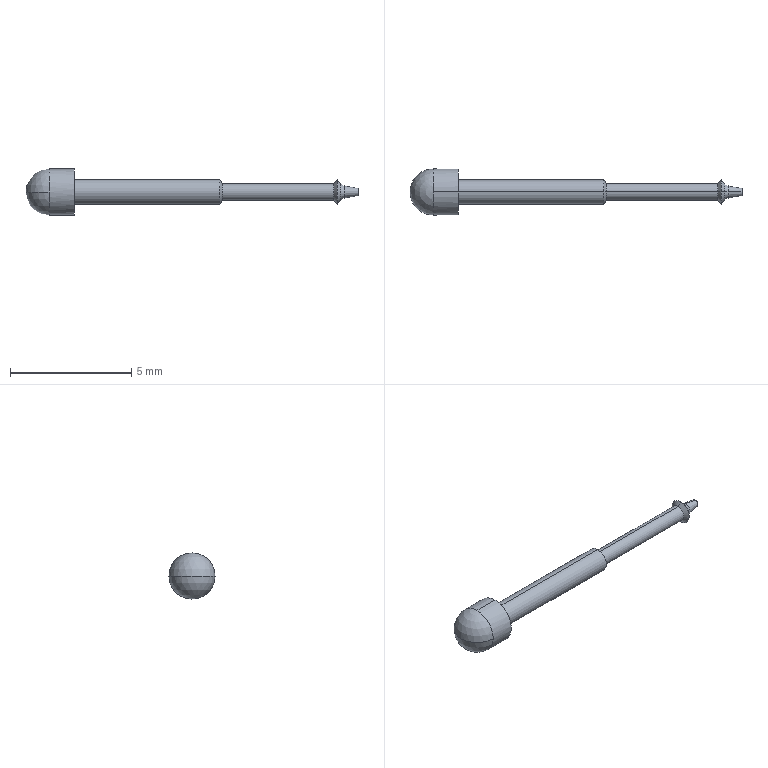Part | STEP file | Shape_NP604_B | 1 solid | 20 faces | box 13.7 x 1.9 x 1.9 mm | volume 11.415 mm3 | cone 10 | cylinder 6 | sphere 2 | plane 2 | commonest cylinder face diameters 0.667 x2 1 x2 1.9 x2
STEP:
#1=CARTESIAN_POINT('',(0.95,0.,-0.95));
#2=VERTEX_POINT('',#1);
#3=CARTESIAN_POINT('',(0.95,-0.95,0.));
#4=VERTEX_POINT('',#3);
#5=CARTESIAN_POINT('',(0.95,0.,0.));
#6=DIRECTION('',(-1.,0.,0.));
#7=DIRECTION('',(0.,0.,1.));
#8=AXIS2_PLACEMENT_3D('',#5,#6,#7);
#9=CIRCLE('',#8,0.95);
#10=EDGE_CURVE('',#2,#4,#9,.T.);
#11=ORIENTED_EDGE('',*,*,#10,.T.);
#12=CARTESIAN_POINT('',(0.,0.,0.));
#13=VERTEX_POINT('',#12);
#14=CARTESIAN_POINT('',(0.95,0.,0.));
#15=DIRECTION('',(0.,0.,-1.));
#16=DIRECTION('',(0.,1.,0.));
#17=AXIS2_PLACEMENT_3D('',#14,#15,#16);
#18=CIRCLE('',#17,0.95);
#19=EDGE_CURVE('',#4,#13,#18,.T.);
#20=ORIENTED_EDGE('',*,*,#19,.T.);
#21=CARTESIAN_POINT('',(0.95,0.95,0.));
#22=VERTEX_POINT('',#21);
#23=CARTESIAN_POINT('',(0.95,0.,0.));
#24=DIRECTION('',(0.,0.,1.));
#25=DIRECTION('',(1.,0.,0.));
#26=AXIS2_PLACEMENT_3D('',#23,#24,#25);
#27=CIRCLE('',#26,0.95);
#28=EDGE_CURVE('',#22,#13,#27,.T.);
#29=ORIENTED_EDGE('',*,*,#28,.F.);
#30=CARTESIAN_POINT('',(0.95,0.,0.));
#31=DIRECTION('',(-1.,0.,0.));
#32=DIRECTION('',(0.,0.,1.));
#33=AXIS2_PLACEMENT_3D('',#30,#31,#32);
#34=CIRCLE('',#33,0.95);
#35=EDGE_CURVE('',#22,#2,#34,.T.);
#36=ORIENTED_EDGE('',*,*,#35,.T.);
#37=EDGE_LOOP('',(#11,#20,#29,#36));
#38=FACE_OUTER_BOUND('',#37,.T.);
#39=CARTESIAN_POINT('',(0.95,0.,0.));
#40=DIRECTION('',(0.,0.,-1.));
#41=DIRECTION('',(0.,1.,0.));
#42=AXIS2_PLACEMENT_3D('',#39,#40,#41);
#43=SPHERICAL_SURFACE('',#42,0.95);
#44=ADVANCED_FACE('',(#38),#43,.T.);
#45=CARTESIAN_POINT('',(13.7,0.,0.1484));
#46=VERTEX_POINT('',#45);
#47=CARTESIAN_POINT('',(13.7,0.,-0.1484));
#48=VERTEX_POINT('',#47);
#49=CARTESIAN_POINT('',(13.7,0.,0.));
#50=DIRECTION('',(-1.,0.,0.));
#51=DIRECTION('',(0.,0.,1.));
#52=AXIS2_PLACEMENT_3D('',#49,#50,#51);
#53=CIRCLE('',#52,0.1484);
#54=EDGE_CURVE('',#46,#48,#53,.T.);
#55=ORIENTED_EDGE('',*,*,#54,.T.);
#56=CARTESIAN_POINT('',(13.124,0.,-0.25));
#57=VERTEX_POINT('',#56);
#58=CARTESIAN_POINT('',(13.7,0.,-0.1484));
#59=DIRECTION('',(-0.9848,0.,-0.1736));
#60=VECTOR('',#59,1000.);
#61=LINE('',#58,#60);
#62=EDGE_CURVE('',#48,#57,#61,.T.);
#63=ORIENTED_EDGE('',*,*,#62,.T.);
#64=CARTESIAN_POINT('',(13.124,0.,0.25));
#65=VERTEX_POINT('',#64);
#66=CARTESIAN_POINT('',(13.124,0.,0.));
#67=DIRECTION('',(-1.,0.,0.));
#68=DIRECTION('',(0.,0.,1.));
#69=AXIS2_PLACEMENT_3D('',#66,#67,#68);
#70=CIRCLE('',#69,0.25);
#71=EDGE_CURVE('',#65,#57,#70,.T.);
#72=ORIENTED_EDGE('',*,*,#71,.F.);
#73=CARTESIAN_POINT('',(13.7,0.,0.1484));
#74=DIRECTION('',(-0.9848,0.,0.1736));
#75=VECTOR('',#74,1000.);
#76=LINE('',#73,#75);
#77=EDGE_CURVE('',#46,#65,#76,.T.);
#78=ORIENTED_EDGE('',*,*,#77,.F.);
#79=EDGE_LOOP('',(#55,#63,#72,#78));
#80=FACE_OUTER_BOUND('',#79,.T.);
#81=CARTESIAN_POINT('',(13.7,0.,0.));
#82=DIRECTION('',(-1.,0.,0.));
#83=DIRECTION('',(0.,0.,1.));
#84=AXIS2_PLACEMENT_3D('',#81,#82,#83);
#85=CONICAL_SURFACE('',#84,0.1484,0.1745);
#86=ADVANCED_FACE('',(#80),#85,.T.);
#87=ORIENTED_EDGE('',*,*,#71,.T.);
#88=CARTESIAN_POINT('',(12.98,0.,-0.3333));
#89=VERTEX_POINT('',#88);
#90=CARTESIAN_POINT('',(13.124,0.,-0.25));
#91=DIRECTION('',(-0.866,0.,-0.5));
#92=VECTOR('',#91,1000.);
#93=LINE('',#90,#92);
#94=EDGE_CURVE('',#57,#89,#93,.T.);
#95=ORIENTED_EDGE('',*,*,#94,.T.);
#96=CARTESIAN_POINT('',(12.98,0.,0.3333));
#97=VERTEX_POINT('',#96);
#98=CARTESIAN_POINT('',(12.98,0.,0.));
#99=DIRECTION('',(-1.,0.,0.));
#100=DIRECTION('',(0.,0.,1.));
#101=AXIS2_PLACEMENT_3D('',#98,#99,#100);
#102=CIRCLE('',#101,0.3333);
#103=EDGE_CURVE('',#97,#89,#102,.T.);
#104=ORIENTED_EDGE('',*,*,#103,.F.);
#105=CARTESIAN_POINT('',(13.124,0.,0.25));
#106=DIRECTION('',(-0.866,0.,0.5));
#107=VECTOR('',#106,1000.);
#108=LINE('',#105,#107);
#109=EDGE_CURVE('',#65,#97,#108,.T.);
#110=ORIENTED_EDGE('',*,*,#109,.F.);
#111=EDGE_LOOP('',(#87,#95,#104,#110));
#112=FACE_OUTER_BOUND('',#111,.T.);
#113=CARTESIAN_POINT('',(13.124,0.,0.));
#114=DIRECTION('',(-1.,0.,0.));
#115=DIRECTION('',(0.,0.,1.));
#116=AXIS2_PLACEMENT_3D('',#113,#114,#115);
#117=CONICAL_SURFACE('',#116,0.25,0.5236);
#118=ADVANCED_FACE('',(#112),#117,.T.);
#119=ORIENTED_EDGE('',*,*,#103,.T.);
#120=CARTESIAN_POINT('',(12.837,0.,-0.5033));
#121=VERTEX_POINT('',#120);
#122=CARTESIAN_POINT('',(12.98,0.,-0.3333));
#123=DIRECTION('',(-0.6428,0.,-0.766));
#124=VECTOR('',#123,1000.);
#125=LINE('',#122,#124);
#126=EDGE_CURVE('',#89,#121,#125,.T.);
#127=ORIENTED_EDGE('',*,*,#126,.T.);
#128=CARTESIAN_POINT('',(12.837,0.,0.5033));
#129=VERTEX_POINT('',#128);
#130=CARTESIAN_POINT('',(12.837,0.,0.));
#131=DIRECTION('',(-1.,0.,0.));
#132=DIRECTION('',(0.,0.,1.));
#133=AXIS2_PLACEMENT_3D('',#130,#131,#132);
#134=CIRCLE('',#133,0.5033);
#135=EDGE_CURVE('',#129,#121,#134,.T.);
#136=ORIENTED_EDGE('',*,*,#135,.F.);
#137=CARTESIAN_POINT('',(12.98,0.,0.3333));
#138=DIRECTION('',(-0.6428,0.,0.766));
#139=VECTOR('',#138,1000.);
#140=LINE('',#137,#139);
#141=EDGE_CURVE('',#97,#129,#140,.T.);
#142=ORIENTED_EDGE('',*,*,#141,.F.);
#143=EDGE_LOOP('',(#119,#127,#136,#142));
#144=FACE_OUTER_BOUND('',#143,.T.);
#145=CARTESIAN_POINT('',(12.98,0.,0.));
#146=DIRECTION('',(-1.,0.,0.));
#147=DIRECTION('',(0.,0.,1.));
#148=AXIS2_PLACEMENT_3D('',#145,#146,#147);
#149=CONICAL_SURFACE('',#148,0.3333,0.8727);
#150=ADVANCED_FACE('',(#144),#149,.T.);
#151=CARTESIAN_POINT('',(12.694,0.,0.3333));
#152=VERTEX_POINT('',#151);
#153=CARTESIAN_POINT('',(12.694,0.,-0.3333));
#154=VERTEX_POINT('',#153);
#155=CARTESIAN_POINT('',(12.694,0.,0.));
#156=DIRECTION('',(-1.,0.,0.));
#157=DIRECTION('',(0.,0.,1.));
#158=AXIS2_PLACEMENT_3D('',#155,#156,#157);
#159=CIRCLE('',#158,0.3333);
#160=EDGE_CURVE('',#152,#154,#159,.T.);
#161=ORIENTED_EDGE('',*,*,#160,.F.);
#162=CARTESIAN_POINT('',(12.837,0.,0.5033));
#163=DIRECTION('',(0.6428,0.,0.766));
#164=VECTOR('',#163,1000.);
#165=LINE('',#162,#164);
#166=EDGE_CURVE('',#152,#129,#165,.T.);
#167=ORIENTED_EDGE('',*,*,#166,.T.);
#168=ORIENTED_EDGE('',*,*,#135,.T.);
#169=CARTESIAN_POINT('',(12.837,0.,-0.5033));
#170=DIRECTION('',(0.6428,0.,-0.766));
#171=VECTOR('',#170,1000.);
#172=LINE('',#169,#171);
#173=EDGE_CURVE('',#154,#121,#172,.T.);
#174=ORIENTED_EDGE('',*,*,#173,.F.);
#175=EDGE_LOOP('',(#161,#167,#168,#174));
#176=FACE_OUTER_BOUND('',#175,.T.);
#177=CARTESIAN_POINT('',(12.837,0.,0.));
#178=DIRECTION('',(1.,0.,0.));
#179=DIRECTION('',(0.,0.,-1.));
#180=AXIS2_PLACEMENT_3D('',#177,#178,#179);
#181=CONICAL_SURFACE('',#180,0.5033,0.8727);
#182=ADVANCED_FACE('',(#176),#181,.T.);
#183=ORIENTED_EDGE('',*,*,#160,.T.);
#184=CARTESIAN_POINT('',(8.096,0.,-0.3333));
#185=VERTEX_POINT('',#184);
#186=CARTESIAN_POINT('',(13.7,0.,-0.3333));
#187=DIRECTION('',(-1.,0.,0.));
#188=VECTOR('',#187,1000.);
#189=LINE('',#186,#188);
#190=EDGE_CURVE('',#154,#185,#189,.T.);
#191=ORIENTED_EDGE('',*,*,#190,.T.);
#192=CARTESIAN_POINT('',(8.096,0.,0.3333));
#193=VERTEX_POINT('',#192);
#194=CARTESIAN_POINT('',(8.096,0.,0.));
#195=DIRECTION('',(-1.,0.,0.));
#196=DIRECTION('',(0.,0.,1.));
#197=AXIS2_PLACEMENT_3D('',#194,#195,#196);
#198=CIRCLE('',#197,0.3333);
#199=EDGE_CURVE('',#193,#185,#198,.T.);
#200=ORIENTED_EDGE('',*,*,#199,.F.);
#201=CARTESIAN_POINT('',(13.7,0.,0.3333));
#202=DIRECTION('',(-1.,0.,0.));
#203=VECTOR('',#202,1000.);
#204=LINE('',#201,#203);
#205=EDGE_CURVE('',#152,#193,#204,.T.);
#206=ORIENTED_EDGE('',*,*,#205,.F.);
#207=EDGE_LOOP('',(#183,#191,#200,#206));
#208=FACE_OUTER_BOUND('',#207,.T.);
#209=CARTESIAN_POINT('',(13.7,0.,0.));
#210=DIRECTION('',(-1.,0.,0.));
#211=DIRECTION('',(0.,0.,1.));
#212=AXIS2_PLACEMENT_3D('',#209,#210,#211);
#213=CYLINDRICAL_SURFACE('',#212,0.3333);
#214=ADVANCED_FACE('',(#208),#213,.T.);
#215=ORIENTED_EDGE('',*,*,#199,.T.);
#216=CARTESIAN_POINT('',(8.,0.,-0.5));
#217=VERTEX_POINT('',#216);
#218=CARTESIAN_POINT('',(8.096,0.,-0.3333));
#219=DIRECTION('',(-0.5,0.,-0.866));
#220=VECTOR('',#219,1000.);
#221=LINE('',#218,#220);
#222=EDGE_CURVE('',#185,#217,#221,.T.);
#223=ORIENTED_EDGE('',*,*,#222,.T.);
#224=CARTESIAN_POINT('',(8.,0.,0.5));
#225=VERTEX_POINT('',#224);
#226=CARTESIAN_POINT('',(8.,0.,0.));
#227=DIRECTION('',(-1.,0.,0.));
#228=DIRECTION('',(0.,0.,1.));
#229=AXIS2_PLACEMENT_3D('',#226,#227,#228);
#230=CIRCLE('',#229,0.5);
#231=EDGE_CURVE('',#225,#217,#230,.T.);
#232=ORIENTED_EDGE('',*,*,#231,.F.);
#233=CARTESIAN_POINT('',(8.096,0.,0.3333));
#234=DIRECTION('',(-0.5,0.,0.866));
#235=VECTOR('',#234,1000.);
#236=LINE('',#233,#235);
#237=EDGE_CURVE('',#193,#225,#236,.T.);
#238=ORIENTED_EDGE('',*,*,#237,.F.);
#239=EDGE_LOOP('',(#215,#223,#232,#238));
#240=FACE_OUTER_BOUND('',#239,.T.);
#241=CARTESIAN_POINT('',(8.096,0.,0.));
#242=DIRECTION('',(-1.,0.,0.));
#243=DIRECTION('',(0.,0.,1.));
#244=AXIS2_PLACEMENT_3D('',#241,#242,#243);
#245=CONICAL_SURFACE('',#244,0.3333,1.047);
#246=ADVANCED_FACE('',(#240),#245,.T.);
#247=ORIENTED_EDGE('',*,*,#231,.T.);
#248=CARTESIAN_POINT('',(2.,0.,-0.5));
#249=VERTEX_POINT('',#248);
#250=CARTESIAN_POINT('',(13.7,0.,-0.5));
#251=DIRECTION('',(-1.,0.,0.));
#252=VECTOR('',#251,1000.);
#253=LINE('',#250,#252);
#254=EDGE_CURVE('',#217,#249,#253,.T.);
#255=ORIENTED_EDGE('',*,*,#254,.T.);
#256=CARTESIAN_POINT('',(2.,0.,0.5));
#257=VERTEX_POINT('',#256);
#258=CARTESIAN_POINT('',(2.,0.,0.));
#259=DIRECTION('',(-1.,0.,0.));
#260=DIRECTION('',(0.,0.,1.));
#261=AXIS2_PLACEMENT_3D('',#258,#259,#260);
#262=CIRCLE('',#261,0.5);
#263=EDGE_CURVE('',#257,#249,#262,.T.);
#264=ORIENTED_EDGE('',*,*,#263,.F.);
#265=CARTESIAN_POINT('',(13.7,0.,0.5));
#266=DIRECTION('',(-1.,0.,0.));
#267=VECTOR('',#266,1000.);
#268=LINE('',#265,#267);
#269=EDGE_CURVE('',#225,#257,#268,.T.);
#270=ORIENTED_EDGE('',*,*,#269,.F.);
#271=EDGE_LOOP('',(#247,#255,#264,#270));
#272=FACE_OUTER_BOUND('',#271,.T.);
#273=CARTESIAN_POINT('',(13.7,0.,0.));
#274=DIRECTION('',(-1.,0.,0.));
#275=DIRECTION('',(0.,0.,1.));
#276=AXIS2_PLACEMENT_3D('',#273,#274,#275);
#277=CYLINDRICAL_SURFACE('',#276,0.5);
#278=ADVANCED_FACE('',(#272),#277,.T.);
#279=CARTESIAN_POINT('',(2.,0.,0.95));
#280=VERTEX_POINT('',#279);
#281=CARTESIAN_POINT('',(2.,0.,-0.95));
#282=VERTEX_POINT('',#281);
#283=CARTESIAN_POINT('',(2.,0.,0.));
#284=DIRECTION('',(-1.,0.,0.));
#285=DIRECTION('',(0.,0.,1.));
#286=AXIS2_PLACEMENT_3D('',#283,#284,#285);
#287=CIRCLE('',#286,0.95);
#288=EDGE_CURVE('',#280,#282,#287,.T.);
#289=ORIENTED_EDGE('',*,*,#288,.T.);
#290=CARTESIAN_POINT('',(13.7,0.,-0.95));
#291=DIRECTION('',(-1.,0.,0.));
#292=VECTOR('',#291,1000.);
#293=LINE('',#290,#292);
#294=EDGE_CURVE('',#282,#2,#293,.T.);
#295=ORIENTED_EDGE('',*,*,#294,.T.);
#296=ORIENTED_EDGE('',*,*,#35,.F.);
#297=CARTESIAN_POINT('',(0.95,0.,0.95));
#298=VERTEX_POINT('',#297);
#299=CARTESIAN_POINT('',(0.95,0.,0.));
#300=DIRECTION('',(-1.,0.,0.));
#301=DIRECTION('',(0.,0.,1.));
#302=AXIS2_PLACEMENT_3D('',#299,#300,#301);
#303=CIRCLE('',#302,0.95);
#304=EDGE_CURVE('',#298,#22,#303,.T.);
#305=ORIENTED_EDGE('',*,*,#304,.F.);
#306=CARTESIAN_POINT('',(13.7,0.,0.95));
#307=DIRECTION('',(-1.,0.,0.));
#308=VECTOR('',#307,1000.);
#309=LINE('',#306,#308);
#310=EDGE_CURVE('',#280,#298,#309,.T.);
#311=ORIENTED_EDGE('',*,*,#310,.F.);
#312=EDGE_LOOP('',(#289,#295,#296,#305,#311));
#313=FACE_OUTER_BOUND('',#312,.T.);
#314=CARTESIAN_POINT('',(13.7,0.,0.));
#315=DIRECTION('',(-1.,0.,0.));
#316=DIRECTION('',(0.,0.,1.));
#317=AXIS2_PLACEMENT_3D('',#314,#315,#316);
#318=CYLINDRICAL_SURFACE('',#317,0.95);
#319=ADVANCED_FACE('',(#313),#318,.T.);
#320=ORIENTED_EDGE('',*,*,#294,.F.);
#321=CARTESIAN_POINT('',(2.,0.,0.));
#322=DIRECTION('',(-1.,0.,0.));
#323=DIRECTION('',(0.,0.,1.));
#324=AXIS2_PLACEMENT_3D('',#321,#322,#323);
#325=CIRCLE('',#324,0.95);
#326=EDGE_CURVE('',#282,#280,#325,.T.);
#327=ORIENTED_EDGE('',*,*,#326,.T.);
#328=ORIENTED_EDGE('',*,*,#310,.T.);
#329=CARTESIAN_POINT('',(0.95,0.,0.));
#330=DIRECTION('',(-1.,0.,0.));
#331=DIRECTION('',(0.,0.,1.));
#332=AXIS2_PLACEMENT_3D('',#329,#330,#331);
#333=CIRCLE('',#332,0.95);
#334=EDGE_CURVE('',#4,#298,#333,.T.);
#335=ORIENTED_EDGE('',*,*,#334,.F.);
#336=ORIENTED_EDGE('',*,*,#10,.F.);
#337=EDGE_LOOP('',(#320,#327,#328,#335,#336));
#338=FACE_OUTER_BOUND('',#337,.T.);
#339=CARTESIAN_POINT('',(13.7,0.,0.));
#340=DIRECTION('',(-1.,0.,0.));
#341=DIRECTION('',(0.,0.,1.));
#342=AXIS2_PLACEMENT_3D('',#339,#340,#341);
#343=CYLINDRICAL_SURFACE('',#342,0.95);
#344=ADVANCED_FACE('',(#338),#343,.T.);
#345=ORIENTED_EDGE('',*,*,#288,.F.);
#346=ORIENTED_EDGE('',*,*,#326,.F.);
#347=EDGE_LOOP('',(#345,#346));
#348=FACE_OUTER_BOUND('',#347,.T.);
#349=ORIENTED_EDGE('',*,*,#263,.T.);
#350=CARTESIAN_POINT('',(2.,0.,0.));
#351=DIRECTION('',(-1.,0.,0.));
#352=DIRECTION('',(0.,0.,1.));
#353=AXIS2_PLACEMENT_3D('',#350,#351,#352);
#354=CIRCLE('',#353,0.5);
#355=EDGE_CURVE('',#249,#257,#354,.T.);
#356=ORIENTED_EDGE('',*,*,#355,.T.);
#357=EDGE_LOOP('',(#349,#356));
#358=FACE_BOUND('',#357,.T.);
#359=CARTESIAN_POINT('',(2.,0.95,0.));
#360=DIRECTION('',(-1.,0.,0.));
#361=DIRECTION('',(0.,0.,1.));
#362=AXIS2_PLACEMENT_3D('',#359,#360,#361);
#363=PLANE('',#362);
#364=ADVANCED_FACE('',(#348,#358),#363,.F.);
#365=ORIENTED_EDGE('',*,*,#254,.F.);
#366=CARTESIAN_POINT('',(8.,0.,0.));
#367=DIRECTION('',(-1.,0.,0.));
#368=DIRECTION('',(0.,0.,1.));
#369=AXIS2_PLACEMENT_3D('',#366,#367,#368);
#370=CIRCLE('',#369,0.5);
#371=EDGE_CURVE('',#217,#225,#370,.T.);
#372=ORIENTED_EDGE('',*,*,#371,.T.);
#373=ORIENTED_EDGE('',*,*,#269,.T.);
#374=ORIENTED_EDGE('',*,*,#355,.F.);
#375=EDGE_LOOP('',(#365,#372,#373,#374));
#376=FACE_OUTER_BOUND('',#375,.T.);
#377=CARTESIAN_POINT('',(13.7,0.,0.));
#378=DIRECTION('',(-1.,0.,0.));
#379=DIRECTION('',(0.,0.,1.));
#380=AXIS2_PLACEMENT_3D('',#377,#378,#379);
#381=CYLINDRICAL_SURFACE('',#380,0.5);
#382=ADVANCED_FACE('',(#376),#381,.T.);
#383=ORIENTED_EDGE('',*,*,#222,.F.);
#384=CARTESIAN_POINT('',(8.096,0.,0.));
#385=DIRECTION('',(-1.,0.,0.));
#386=DIRECTION('',(0.,0.,1.));
#387=AXIS2_PLACEMENT_3D('',#384,#385,#386);
#388=CIRCLE('',#387,0.3333);
#389=EDGE_CURVE('',#185,#193,#388,.T.);
#390=ORIENTED_EDGE('',*,*,#389,.T.);
#391=ORIENTED_EDGE('',*,*,#237,.T.);
#392=ORIENTED_EDGE('',*,*,#371,.F.);
#393=EDGE_LOOP('',(#383,#390,#391,#392));
#394=FACE_OUTER_BOUND('',#393,.T.);
#395=CARTESIAN_POINT('',(8.096,0.,0.));
#396=DIRECTION('',(-1.,0.,0.));
#397=DIRECTION('',(0.,0.,1.));
#398=AXIS2_PLACEMENT_3D('',#395,#396,#397);
#399=CONICAL_SURFACE('',#398,0.3333,1.047);
#400=ADVANCED_FACE('',(#394),#399,.T.);
#401=ORIENTED_EDGE('',*,*,#190,.F.);
#402=CARTESIAN_POINT('',(12.694,0.,0.));
#403=DIRECTION('',(-1.,0.,0.));
#404=DIRECTION('',(0.,0.,1.));
#405=AXIS2_PLACEMENT_3D('',#402,#403,#404);
#406=CIRCLE('',#405,0.3333);
#407=EDGE_CURVE('',#154,#152,#406,.T.);
#408=ORIENTED_EDGE('',*,*,#407,.T.);
#409=ORIENTED_EDGE('',*,*,#205,.T.);
#410=ORIENTED_EDGE('',*,*,#389,.F.);
#411=EDGE_LOOP('',(#401,#408,#409,#410));
#412=FACE_OUTER_BOUND('',#411,.T.);
#413=CARTESIAN_POINT('',(13.7,0.,0.));
#414=DIRECTION('',(-1.,0.,0.));
#415=DIRECTION('',(0.,0.,1.));
#416=AXIS2_PLACEMENT_3D('',#413,#414,#415);
#417=CYLINDRICAL_SURFACE('',#416,0.3333);
#418=ADVANCED_FACE('',(#412),#417,.T.);
#419=ORIENTED_EDGE('',*,*,#166,.F.);
#420=ORIENTED_EDGE('',*,*,#407,.F.);
#421=ORIENTED_EDGE('',*,*,#173,.T.);
#422=CARTESIAN_POINT('',(12.837,0.,0.));
#423=DIRECTION('',(-1.,0.,0.));
#424=DIRECTION('',(0.,0.,1.));
#425=AXIS2_PLACEMENT_3D('',#422,#423,#424);
#426=CIRCLE('',#425,0.5033);
#427=EDGE_CURVE('',#121,#129,#426,.T.);
#428=ORIENTED_EDGE('',*,*,#427,.T.);
#429=EDGE_LOOP('',(#419,#420,#421,#428));
#430=FACE_OUTER_BOUND('',#429,.T.);
#431=CARTESIAN_POINT('',(12.837,0.,0.));
#432=DIRECTION('',(1.,0.,0.));
#433=DIRECTION('',(0.,0.,-1.));
#434=AXIS2_PLACEMENT_3D('',#431,#432,#433);
#435=CONICAL_SURFACE('',#434,0.5033,0.8727);
#436=ADVANCED_FACE('',(#430),#435,.T.);
#437=ORIENTED_EDGE('',*,*,#126,.F.);
#438=CARTESIAN_POINT('',(12.98,0.,0.));
#439=DIRECTION('',(-1.,0.,0.));
#440=DIRECTION('',(0.,0.,1.));
#441=AXIS2_PLACEMENT_3D('',#438,#439,#440);
#442=CIRCLE('',#441,0.3333);
#443=EDGE_CURVE('',#89,#97,#442,.T.);
#444=ORIENTED_EDGE('',*,*,#443,.T.);
#445=ORIENTED_EDGE('',*,*,#141,.T.);
#446=ORIENTED_EDGE('',*,*,#427,.F.);
#447=EDGE_LOOP('',(#437,#444,#445,#446));
#448=FACE_OUTER_BOUND('',#447,.T.);
#449=CARTESIAN_POINT('',(12.98,0.,0.));
#450=DIRECTION('',(-1.,0.,0.));
#451=DIRECTION('',(0.,0.,1.));
#452=AXIS2_PLACEMENT_3D('',#449,#450,#451);
#453=CONICAL_SURFACE('',#452,0.3333,0.8727);
#454=ADVANCED_FACE('',(#448),#453,.T.);
#455=ORIENTED_EDGE('',*,*,#94,.F.);
#456=CARTESIAN_POINT('',(13.124,0.,0.));
#457=DIRECTION('',(-1.,0.,0.));
#458=DIRECTION('',(0.,0.,1.));
#459=AXIS2_PLACEMENT_3D('',#456,#457,#458);
#460=CIRCLE('',#459,0.25);
#461=EDGE_CURVE('',#57,#65,#460,.T.);
#462=ORIENTED_EDGE('',*,*,#461,.T.);
#463=ORIENTED_EDGE('',*,*,#109,.T.);
#464=ORIENTED_EDGE('',*,*,#443,.F.);
#465=EDGE_LOOP('',(#455,#462,#463,#464));
#466=FACE_OUTER_BOUND('',#465,.T.);
#467=CARTESIAN_POINT('',(13.124,0.,0.));
#468=DIRECTION('',(-1.,0.,0.));
#469=DIRECTION('',(0.,0.,1.));
#470=AXIS2_PLACEMENT_3D('',#467,#468,#469);
#471=CONICAL_SURFACE('',#470,0.25,0.5236);
#472=ADVANCED_FACE('',(#466),#471,.T.);
#473=ORIENTED_EDGE('',*,*,#62,.F.);
#474=CARTESIAN_POINT('',(13.7,0.,0.));
#475=DIRECTION('',(-1.,0.,0.));
#476=DIRECTION('',(0.,0.,1.));
#477=AXIS2_PLACEMENT_3D('',#474,#475,#476);
#478=CIRCLE('',#477,0.1484);
#479=EDGE_CURVE('',#48,#46,#478,.T.);
#480=ORIENTED_EDGE('',*,*,#479,.T.);
#481=ORIENTED_EDGE('',*,*,#77,.T.);
#482=ORIENTED_EDGE('',*,*,#461,.F.);
#483=EDGE_LOOP('',(#473,#480,#481,#482));
#484=FACE_OUTER_BOUND('',#483,.T.);
#485=CARTESIAN_POINT('',(13.7,0.,0.));
#486=DIRECTION('',(-1.,0.,0.));
#487=DIRECTION('',(0.,0.,1.));
#488=AXIS2_PLACEMENT_3D('',#485,#486,#487);
#489=CONICAL_SURFACE('',#488,0.1484,0.1745);
#490=ADVANCED_FACE('',(#484),#489,.T.);
#491=ORIENTED_EDGE('',*,*,#54,.F.);
#492=ORIENTED_EDGE('',*,*,#479,.F.);
#493=EDGE_LOOP('',(#491,#492));
#494=FACE_OUTER_BOUND('',#493,.T.);
#495=CARTESIAN_POINT('',(13.7,0.1484,0.));
#496=DIRECTION('',(-1.,0.,0.));
#497=DIRECTION('',(0.,0.,1.));
#498=AXIS2_PLACEMENT_3D('',#495,#496,#497);
#499=PLANE('',#498);
#500=ADVANCED_FACE('',(#494),#499,.F.);
#501=ORIENTED_EDGE('',*,*,#19,.F.);
#502=ORIENTED_EDGE('',*,*,#334,.T.);
#503=ORIENTED_EDGE('',*,*,#304,.T.);
#504=ORIENTED_EDGE('',*,*,#28,.T.);
#505=EDGE_LOOP('',(#501,#502,#503,#504));
#506=FACE_OUTER_BOUND('',#505,.T.);
#507=CARTESIAN_POINT('',(0.95,0.,0.));
#508=DIRECTION('',(0.,0.,-1.));
#509=DIRECTION('',(0.,1.,0.));
#510=AXIS2_PLACEMENT_3D('',#507,#508,#509);
#511=SPHERICAL_SURFACE('',#510,0.95);
#512=ADVANCED_FACE('',(#506),#511,.T.);
#513=CLOSED_SHELL('',(#44,#86,#118,#150,#182,#214,#246,#278,#319,#344,#364,#382,#400,#418,#436,#454,#472,#490,#500,#512));
#514=MANIFOLD_SOLID_BREP('',#513);
#515=CARTESIAN_POINT('',(0.,0.,0.));
#516=DIRECTION('',(0.,0.,1.));
#517=DIRECTION('',(1.,0.,0.));
#518=AXIS2_PLACEMENT_3D('',#515,#516,#517);
#519=(LENGTH_UNIT()NAMED_UNIT(*)SI_UNIT(.MILLI.,.METRE.));
#520=UNCERTAINTY_MEASURE_WITH_UNIT(LENGTH_MEASURE(0.00001),#519,'','');
#521=(NAMED_UNIT(*)PLANE_ANGLE_UNIT()SI_UNIT($,.RADIAN.));
#522=(NAMED_UNIT(*)SI_UNIT($,.STERADIAN.)SOLID_ANGLE_UNIT());
#523=(GEOMETRIC_REPRESENTATION_CONTEXT(3)GLOBAL_UNCERTAINTY_ASSIGNED_CONTEXT((#520))GLOBAL_UNIT_ASSIGNED_CONTEXT((#519,#521,#522))REPRESENTATION_CONTEXT('',''));
#524=ADVANCED_BREP_SHAPE_REPRESENTATION('',(#514,#518),#523);